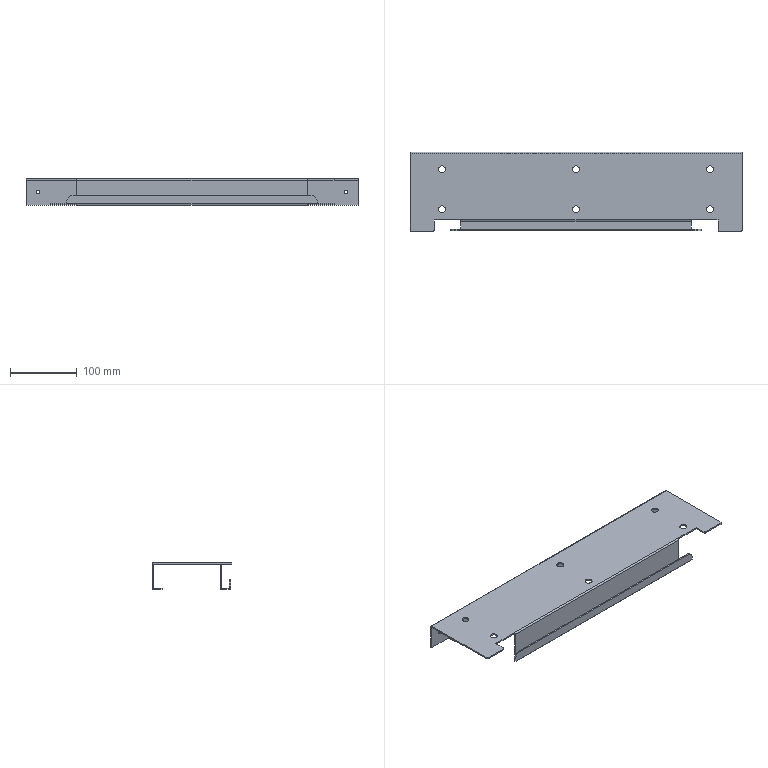Part | STEP file | SX-022-02 | 1 solid | 84 faces | box 498 x 120 x 40 mm | volume 196950 mm3 | plane 50 | cylinder 34 | commonest cylinder face diameters 10.5 x12 5.4 x6 0.4 x5 4.4 x5 4 x4 20 x2